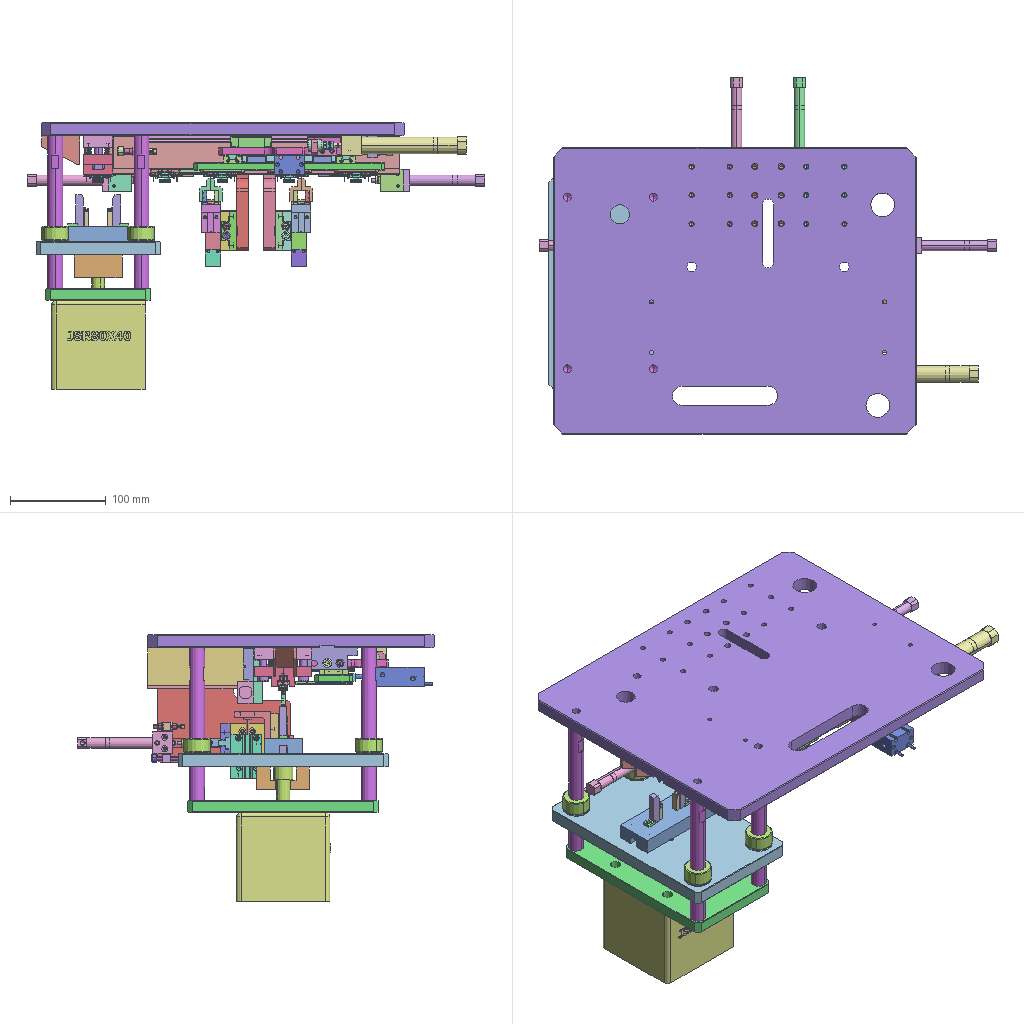Assembly | STEP file | 119 different items | 282 placed | box 479 x 373 x 279 mm
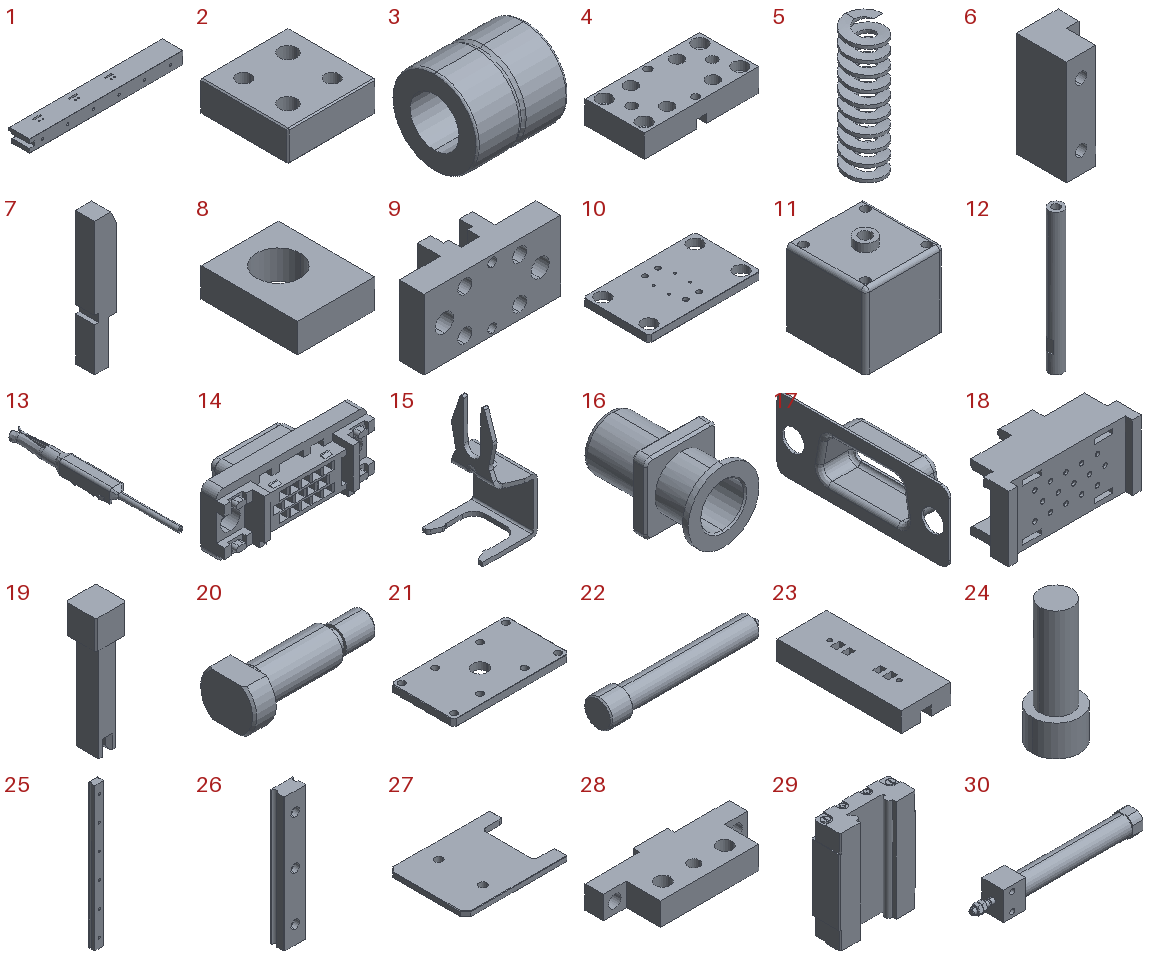Parts list (item | name | quantity | parent item | size | volume):
1 | Semi-finished track | x1 | in Assembly | 300 x 40 x 24 mm | 231580 mm3
2 | A037 | x2 | in Assembly | 20 x 20 x 7 mm | 2500 mm3
3 | LMUT16 | x4 | in Riveting rivet station | 29.9 x 28 x 28 mm | 12313 mm3
4 | Riveting base | x1 | in Riveting rivet station | 60 x 30.8 x 12 mm | 18745 mm3
5 | SWF6-20 spring | x4 | in Riveting rivet station | 6 x 6 x 20 mm | 104.246 mm3
6 | Large cylinder connector mounting block | x2 | in Riveting rivet station | 20 x 24 x 50 mm | 18141 mm3
7 | Riveting product locating pin | x2 | in Riveting rivet station | 8 x 7 x 49 mm | 2346 mm3
8 | Stopper plate | x2 | in Riveting rivet station | 8 x 10 x 3 mm | 192.287 mm3
9 | Riveting floating block | x1 | in Riveting rivet station | 60 x 20.8 x 30.8 mm | 21870 mm3
10 | Riveting slide mounting plate | x1 | in Riveting rivet station | 220 x 130 x 14 mm | 361910 mm3
11 | JSR80X40 | x1 | in Riveting rivet station | 99 x 98 x 103.5 mm | 861667 mm3
12 | Guide pillar | x4 | in Riveting rivet station | 16 x 16 x 160 mm | 28723 mm3
13 | CONTACT | x75 | - | 1.85 x 19.165 x 1.65 mm | 9.871 mm3
14 | HOUSING | x5 | - | 30.8 x 13.55 x 12.55 mm | 1641 mm3
15 | LATCH | x10 | - | 4.62 x 5.1 x 10 mm | 18.37 mm3
16 | MAODING | x10 | - | 5 x 8 x 5 mm | 51.782 mm3
17 | SHELL | x5 | - | 6.2 x 30.8 x 12.55 mm | 200.201 mm3
18 | COVER | x5 | - | 19.4 x 8.9 x 9.6 mm | 433.37 mm3
19 | Riveting press block | x2 | in Riveting rivet station | 8.5 x 8.5 x 35.35 mm | 1342 mm3
20 | CLBDG8-18 | x2 | in Riveting rivet station | 32 x 13 x 10 mm | 1712 mm3
21 | Large cylinder base plate | x1 | in Riveting rivet station | 200 x 110 x 12 mm | 247760 mm3
22 | Riveting punch | x2 | in Riveting rivet station | 28.754 x 5 x 5 mm | 342.473 mm3
23 | Riveting upper die seat | x1 | in Riveting rivet station | 40 x 100 x 16 mm | 55230 mm3
24 | M14 screw | x1 | in Riveting rivet station | 20.67 x 20.67 x 53.57 mm | 10711 mm3
25 | 1SE2BZ16-230 | x1 | in Assembly | 15 x 9.5 x 230 mm | 29723 mm3
26 | SEBZ10-551 | x2 | in Assembly | 9 x 5.5 x 55 mm | 2176 mm3
27 | A039 | x2 | in Assembly | 60 x 46 x 3 mm | 7033 mm3
28 | Stopper buffer seat | x2 | in Assembly | 63 x 26 x 10 mm | 10700 mm3
29 | 2SE2BZ16-230 | x1 | in Assembly | 32 x 12 x 42.4 mm | 12424 mm3
30 | CJ2RA16-75(0_0_0) | x1 | in Assembly | - | -
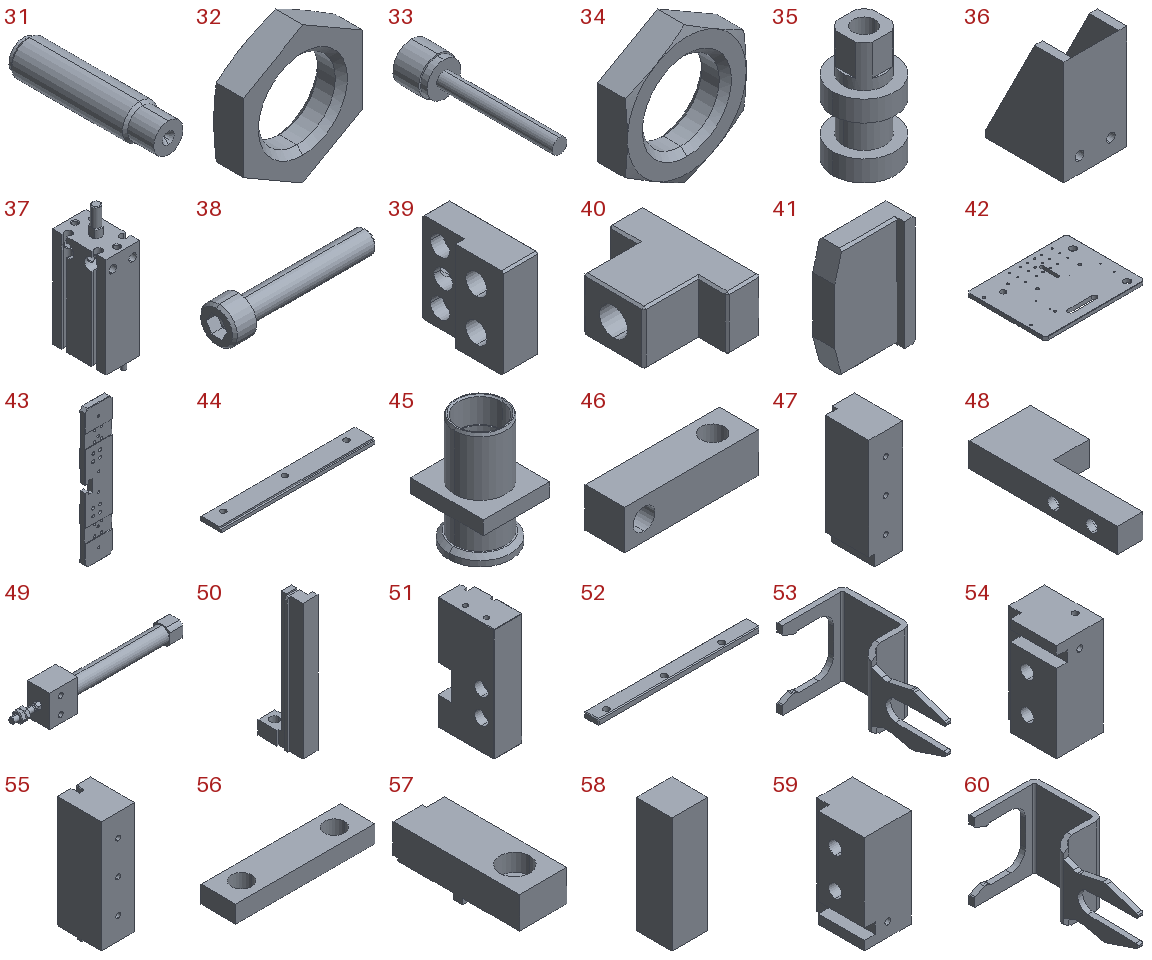31 | MAKC0604A1 | x4 | in MAKC0604A | 6 x 25 x 6 mm | 609.83 mm3
32 | MAKC0604A4 | x4 | in MAKC0604A | 8 x 2 x 9.238 mm | 65.48 mm3
33 | MAKC0604A2 | x4 | in MAKC0604A | 4.6 x 18.25 x 4.6 mm | 100.526 mm3
34 | MAKC0604A3 | x4 | in MAKC0604A | 8 x 2 x 9.238 mm | 65.48 mm3
35 | Product shift T-head | x1 | in Assembly | 12 x 12 x 22 mm | 1377 mm3
36 | Discharge hopper | x1 | in Assembly | 24 x 30 x 40 mm | 12073 mm3
37 | CDU16-20D-A93 (0) | x1 | in Assembly | 20 x 32 x 85 mm | 33757 mm3
38 | CB6-35 | x2 | in Assembly | 41 x 10 x 10 mm | 1382 mm3
39 | Brake spring-press seat | x3 | in Assembly | 6 x 15 x 15 mm | 832.507 mm3
40 | A036 | x1 | in Assembly | 13 x 17.5 x 8 mm | 1094 mm3
41 | Brake block | x3 | in Assembly | 10 x 4 x 15 mm | 442.73 mm3
42 | Base plate | x1 | in Assembly | 380 x 300 x 14 mm | 1501141 mm3
43 | A034 | x1 | in Assembly | 40 x 8 x 200 mm | 52528 mm3
44 | Feed slide cover_Default | x2 | in Rivet-harpoon feed and assembly | 100 x 13 x 3 mm | 3712 mm3
45 | Rivet_Default | x3 | in Rivet-harpoon feed and assembly | 4.8 x 5.3 x 8.1 mm | 41.537 mm3
46 | Optical fiber mount | x1 | in Rivet-harpoon feed and assembly | 20.5 x 6 x 6 mm | 628.955 mm3
47 | Harpoon feed slide_Default | x1 | in Rivet-harpoon feed and assembly | 30 x 42.8 x 100 mm | 120679 mm3
48 | Rivet air-suction cylinder seat | x1 | in Rivet-harpoon feed and assembly | 24 x 58 x 9.55 mm | 7786 mm3
49 | CJ2RKA10-45(0_0_0) | x2 | in Rivet-harpoon feed and assembly, Rivet-harpoon shift assembly | - | -
50 | Rivet push rod_Default | x1 | in Rivet-harpoon feed and assembly | 6.34 x 16 x 50 mm | 1914 mm3
51 | Rivet push-in slide_Default | x1 | in Rivet-harpoon feed and assembly | 20 x 40 x 80 mm | 57141 mm3
52 | Harpoon track cover plate_Default | x1 | in Rivet-harpoon feed and assembly | 98 x 8.5 x 3.6 mm | 2841 mm3
53 | Harpoon_Default | x2 | in Rivet-harpoon feed and assembly | 4.47 x 10 x 5.3 mm | 19.521 mm3
54 | Rivet press-in harpoon track_Default | x1 | in Rivet-harpoon feed and assembly | 20 x 25 x 42 mm | 18009 mm3
55 | Rivet feed slide_Default | x1 | in Rivet-harpoon feed and assembly | 30 x 39.6 x 101.8 mm | 114670 mm3
56 | Spring stop block | x3 | in Rivet-harpoon feed and assembly, Mirror rivet-harpoon feed and assembly, Assembly | 24 x 6 x 3 mm | 374.273 mm3
57 | Rivet push-in slide2_Default | x1 | in Rivet-harpoon feed and assembly | 15 x 40 x 11.8 mm | 5491 mm3
58 | Harpoon track spring pin | x1 | in Rivet-harpoon feed and assembly | 4.58 x 4.58 x 15 mm | 314.646 mm3
59 | Mirror rivet press-in harpoon track_Default | x1 | in Mirror rivet-harpoon feed and assembly | 20 x 25 x 42 mm | 18009 mm3
60 | Mirror harpoon_Default | x2 | in Mirror rivet-harpoon feed and assembly | 4.47 x 10 x 5.3 mm | 19.521 mm3
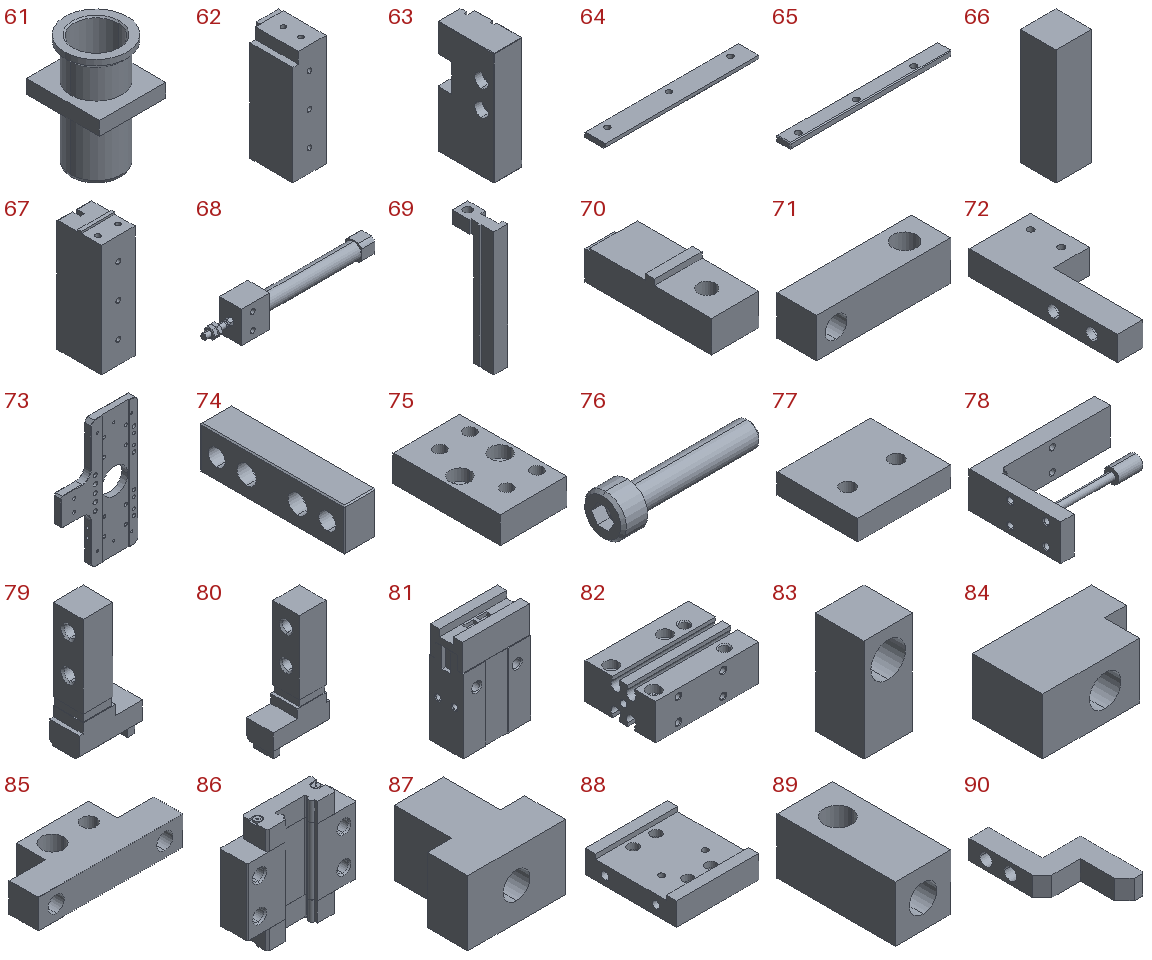61 | Mirror rivet_Default | x3 | in Mirror rivet-harpoon feed and assembly | 4.8 x 5.3 x 8.1 mm | 41.537 mm3
62 | Mirror harpoon feed slide_Default | x1 | in Mirror rivet-harpoon feed and assembly | 30 x 42.8 x 100 mm | 120679 mm3
63 | Mirror rivet push-in slide_Default | x1 | in Mirror rivet-harpoon feed and assembly | 20 x 40 x 80 mm | 57141 mm3
64 | Mirror feed slide cover_Default | x2 | in Mirror rivet-harpoon feed and assembly | 100 x 13 x 3 mm | 3712 mm3
65 | Mirror harpoon track cover plate_Default | x1 | in Mirror rivet-harpoon feed and assembly | 98 x 8.5 x 3.6 mm | 2841 mm3
66 | Mirror harpoon track spring pin | x1 | in Mirror rivet-harpoon feed and assembly | 4.58 x 4.58 x 15 mm | 314.646 mm3
67 | Mirror rivet feed slide_Default | x1 | in Mirror rivet-harpoon feed and assembly | 30 x 39.6 x 101.8 mm | 114670 mm3
68 | Mirror CJ2RKA10-45(0_0_0) | x1 | in Mirror rivet-harpoon feed and assembly | 119 x 16 x 23 mm | 12263 mm3
69 | Mirror rivet push rod_Default | x1 | in Mirror rivet-harpoon feed and assembly | 6.34 x 16 x 50 mm | 1914 mm3
70 | Mirror rivet push-in slide2_Default | x1 | in Mirror rivet-harpoon feed and assembly | 15 x 40 x 11.8 mm | 5491 mm3
71 | Mirror optical fiber mount | x1 | in Mirror rivet-harpoon feed and assembly | 20.5 x 6 x 6 mm | 628.955 mm3
72 | Mirror rivet air-suction cylinder seat | x1 | in Mirror rivet-harpoon feed and assembly | 24 x 58 x 9.55 mm | 7786 mm3
73 | A033 | x1 | in Assembly | 90 x 8 x 148 mm | 59811 mm3
74 | A038 | x2 | in Assembly | 7.5 x 34 x 10 mm | 1805 mm3
75 | Gripper cylinder connecting plate | x1 | in Rivet-harpoon shift assembly | 20 x 32 x 8 mm | 4330 mm3
76 | CBAL5-25 | x2 | in Rivet-harpoon shift assembly | 30 x 8.5 x 8.5 mm | 731.85 mm3
77 | Shift cylinder pad | x1 | in Rivet-harpoon shift assembly | 23 x 20 x 5 mm | 2204 mm3
78 | MXH6-15-b | x1 | in Rivet-harpoon shift assembly | 52 x 38 x 15 mm | 8036 mm3
79 | 2 | x1 | in MHZA2-6D | 8.45 x 4 x 17.2 mm | 295.775 mm3
80 | 3 | x1 | in MHZA2-6D | 8.45 x 4 x 17.2 mm | 295.775 mm3
81 | 1 | x1 | in MHZA2-6D | 20 x 10 x 29.8 mm | 5405 mm3
82 | MXH6-15-a | x1 | in Rivet-harpoon shift assembly | 46 x 31.7 x 16 mm | 17954 mm3
83 | Buffer mount | x1 | in Rivet-harpoon shift assembly | 8.5 x 8.5 x 18 mm | 935.428 mm3
84 | Shift T-head fixing seat | x2 | in Rivet-harpoon shift assembly | 16.9 x 10 x 8 mm | 941.722 mm3
85 | Harpoon shift buffer fixing seat | x1 | in Rivet-harpoon shift assembly | 40 x 16 x 8 mm | 2986 mm3
86 | Linear slider | x1 | in Rivet-harpoon shift assembly | 31 x 7.8 x 30 mm | 4960 mm3
87 | Shift T-type connector | x1 | in Rivet-harpoon shift assembly | 12 x 12 x 8 mm | 713.364 mm3
88 | Slide cylinder mount | x1 | in Rivet-harpoon shift assembly | 36 x 40 x 10 mm | 10816 mm3
89 | Stopper | x1 | in Rivet-harpoon shift assembly | 8.5 x 18 x 8.5 mm | 1038 mm3
90 | Gripper_Default | x2 | in Rivet-harpoon shift assembly | 11.85 x 24 x 4 mm | 454.253 mm3
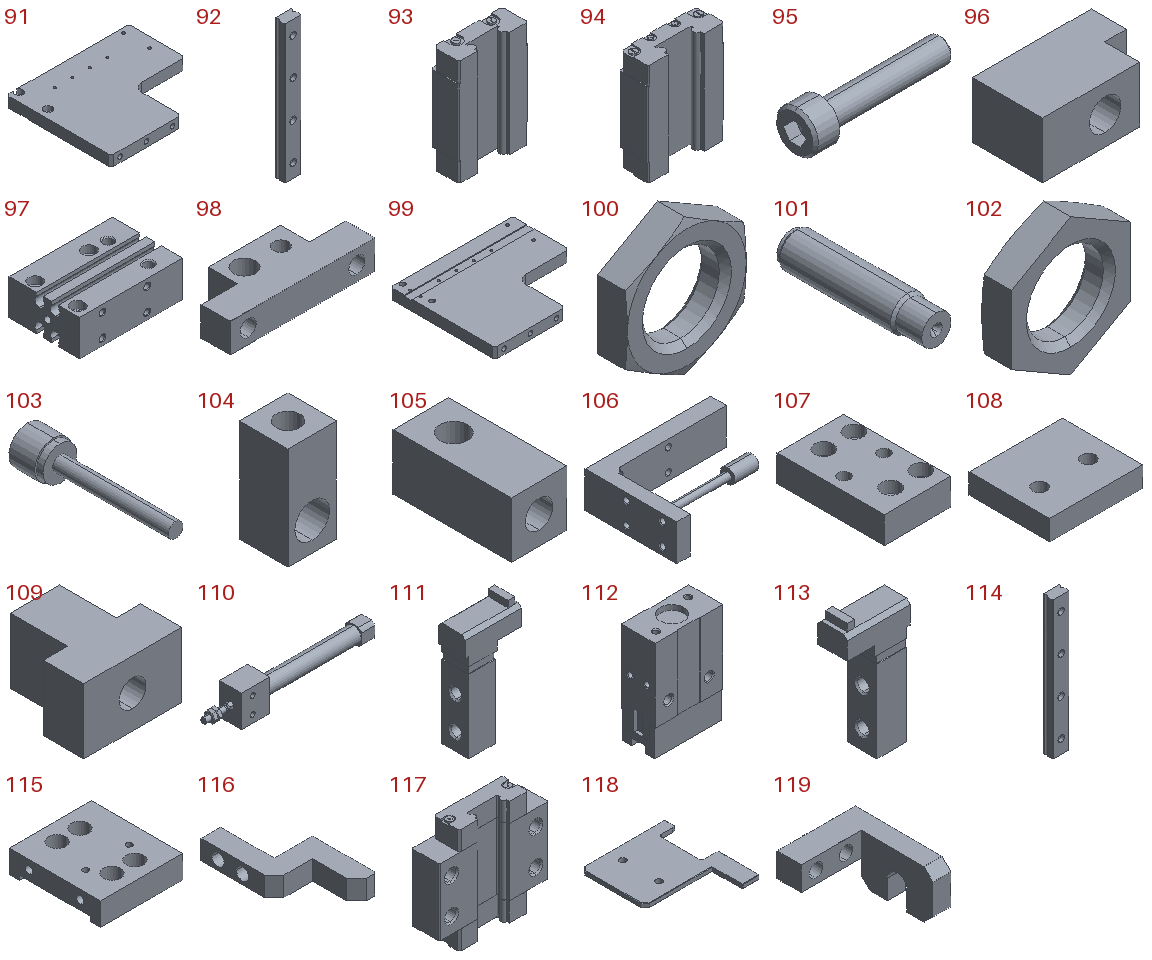91 | Shift support plate_Default | x1 | in Rivet-harpoon shift assembly | 140 x 120 x 12 mm | 158109 mm3
92 | Linear rail | x1 | in Rivet-harpoon shift assembly | 9 x 5.5 x 75 mm | 3056 mm3
93 | SEBZ10-552 | x2 | in Assembly | 20 x 7.8 x 30 mm | 3537 mm3
94 | 3SE2BZ16-230 | x1 | in Assembly | 32 x 12 x 42.4 mm | 12424 mm3
95 | Mirror CBAL5-25 | x2 | in Mirror rivet-harpoon shift assembly | 30 x 8.5 x 8.5 mm | 731.85 mm3
96 | Mirror shift T-head fixing seat | x2 | in Mirror rivet-harpoon shift assembly | 16.9 x 10 x 8 mm | 941.722 mm3
97 | Mirror MXH6-15-a | x1 | in Mirror rivet-harpoon shift assembly | 46 x 31.7 x 16 mm | 17954 mm3
98 | Mirror harpoon shift buffer fixing seat | x1 | in Mirror rivet-harpoon shift assembly | 40 x 16 x 8 mm | 2986 mm3
99 | Mirror shift support plate_Default | x1 | in Mirror rivet-harpoon shift assembly | 140 x 120 x 12 mm | 158109 mm3
100 | Mirror MAKC0604A3 | x2 | in 101, Mirror MAKC0604A | 8 x 2 x 9.238 mm | 65.48 mm3
101 | Mirror MAKC0604A1 | x2 | in 101, Mirror MAKC0604A | 6 x 25 x 6 mm | 609.83 mm3
102 | Mirror MAKC0604A4 | x2 | in 101, Mirror MAKC0604A | 8 x 2 x 9.238 mm | 65.48 mm3
103 | Mirror MAKC0604A2 | x2 | in 101, Mirror MAKC0604A | 4.6 x 18.25 x 4.6 mm | 100.526 mm3
104 | Mirror buffer mount | x1 | in Mirror rivet-harpoon shift assembly | 8.5 x 8.5 x 18 mm | 935.428 mm3
105 | Mirror stopper | x1 | in Mirror rivet-harpoon shift assembly | 8.5 x 18 x 8.5 mm | 1038 mm3
106 | Mirror MXH6-15-b | x1 | in Mirror rivet-harpoon shift assembly | 52 x 38 x 15 mm | 8036 mm3
107 | Mirror gripper cylinder connecting plate | x1 | in Mirror rivet-harpoon shift assembly | 20 x 32 x 8 mm | 4330 mm3
108 | Mirror shift cylinder pad | x1 | in Mirror rivet-harpoon shift assembly | 23 x 20 x 5 mm | 2204 mm3
109 | Mirror shift T-type connector | x1 | in Mirror rivet-harpoon shift assembly | 12 x 12 x 8 mm | 713.364 mm3
110 | Mirror CJ2RKA10-45(0_0_0)1 | x1 | in Mirror rivet-harpoon shift assembly | 119 x 16 x 23 mm | 12263 mm3
111 | Mirror2 | x1 | in Mirror MHZA2-6D | 8.45 x 4 x 17.2 mm | 295.775 mm3
112 | Mirror1 | x1 | in Mirror MHZA2-6D | 20 x 10 x 29.8 mm | 5405 mm3
113 | Mirror3 | x1 | in Mirror MHZA2-6D | 8.45 x 4 x 17.2 mm | 295.775 mm3
114 | Mirror linear rail | x1 | in Mirror rivet-harpoon shift assembly | 9 x 5.5 x 75 mm | 3056 mm3
115 | Mirror slide cylinder mount | x1 | in Mirror rivet-harpoon shift assembly | 36 x 40 x 10 mm | 10816 mm3
116 | Mirror gripper_Default | x2 | in Mirror rivet-harpoon shift assembly | 11.85 x 24 x 4 mm | 454.253 mm3
117 | Mirror linear slider | x1 | in Mirror rivet-harpoon shift assembly | 31 x 7.8 x 30 mm | 4960 mm3
118 | Riveting station pick claw | x1 | in Assembly | 60 x 67.74 x 3 mm | 7814 mm3
119 | Product shift cylinder connector | x1 | in Assembly | 26 x 32 x 16 mm | 3279 mm3
Placements (level | parent | child | x y z in mm | rotation matrix by rows):
1 | Assembly | Semi-finished track | -101.117 -51.384 -17.0 | 1 0 0 0 0 1 0 -1 0
1 | Assembly | A037 | 33.992 -10.639 -35.0 | -1 0 0 0 -1 0 0 0 1
1 | Assembly | Riveting rivet station | -113.758 -35.953 -13.0 | 0 -1 0 -1 0 0 0 0 -1
2 | Riveting rivet station | LMUT16 | -86.569 -42.241 118.75 | 0 -0.8149 0.5796 0 0.5796 0.8149 -1 0 0
2 | Riveting rivet station | Riveting base | -26.539 -12.691 -6.0 | 1 0 0 0 1 0 0 0 1
2 | Riveting rivet station | SWF6-20 spring | -8.595 -6.448 -1.8 | 0.2253 0.9743 0 -0.9743 0.2253 0 0 0 1
2 | Riveting rivet station | Large cylinder connector mounting block | -4.069 27.759 118.65 | 1 0 0 0 0 -1 0 1 -0
2 | Riveting rivet station | Riveting product locating pin | 7.931 26.204 104.65 | 0 -1 0 -1 0 0 0 0 -1
2 | Riveting rivet station | Stopper plate | 7.931 -21.612 85.65 | -1 0 0 0 -1 0 0 0 1
2 | Riveting rivet station | Riveting floating block | -26.539 18.109 14.0 | 1 0 0 0 0 -1 0 1 0
2 | Riveting rivet station | Riveting slide mounting plate | -106.569 -62.241 104.65 | 1 0 0 0 1 0 0 0 1
2 | Riveting rivet station | Stopper plate | -0.069 27.129 85.65 | 1 0 0 0 1 0 0 0 1
2 | Riveting rivet station | Riveting product locating pin | -1.069 -20.686 104.65 | 0 1 0 1 0 0 0 0 -1
2 | Riveting rivet station | JSR80X40 | 3.431 2.759 210.5 | 1 0 0 0 -1 0 0 0 -1
2 | Riveting rivet station | LMUT16 | 93.431 -42.241 118.75 | 0 -0.8149 0.5796 0 0.5796 0.8149 -1 0 0
2 | Riveting rivet station | Guide pillar | -86.569 -42.241 -6.0 | 1 0 0 0 1 0 0 0 1
2 | Riveting rivet station | SWF6-20 spring | 15.405 12.352 -1.8 | 0.2253 0.9743 0 -0.9743 0.2253 0 0 0 1
2 | Riveting rivet station | subassembly 2 | 9.711 18.109 36.35 | 0 0 1 -1 0 0 0 -1 0
3 | subassembly 2 | CONTACT | 20.235 -6.585 -8.205 | 1 0 0 0 1 0 0 0 1
3 | subassembly 2 | CONTACT | 12.22 -6.585 -6.225 | 1 0 0 0 1 0 0 0 1
3 | subassembly 2 | HOUSING | 15.4 7.3 -6.275 | 1 0 0 0 1 0 0 0 1
3 | subassembly 2 | CONTACT | 16.8 -6.585 -6.225 | 1 0 0 0 1 0 0 0 1
3 | subassembly 2 | CONTACT | 15.655 -6.585 -4.245 | 1 0 0 0 1 0 0 0 1
3 | subassembly 2 | LATCH | 2.73 -0.15 -6.275 | 1 0 0 0 0 -1 0 1 0
3 | subassembly 2 | CONTACT | 14.51 -6.585 -6.225 | 1 0 0 0 1 0 0 0 1
3 | subassembly 2 | CONTACT | 9.93 -6.585 -6.225 | 1 0 0 0 1 0 0 0 1
3 | subassembly 2 | CONTACT | 13.365 -6.585 -4.245 | 1 0 0 0 1 0 0 0 1
3 | subassembly 2 | CONTACT | 19.09 -6.585 -6.225 | 1 0 0 0 1 0 0 0 1
3 | subassembly 2 | MAODING | 27.895 -0.15 -6.275 | 1 0 0 0 1 0 0 0 1
3 | subassembly 2 | SHELL | 15.4 7.7 -10.275 | 0 1 0 1 0 0 0 0 -1
3 | subassembly 2 | CONTACT | 11.075 -6.585 -4.245 | 1 0 0 0 1 0 0 0 1
3 | subassembly 2 | CONTACT | 17.945 -6.585 -8.205 | 1 0 0 0 1 0 0 0 1
3 | subassembly 2 | CONTACT | 11.075 -6.585 -8.205 | 1 0 0 0 1 0 0 0 1
3 | subassembly 2 | CONTACT | 20.235 -6.585 -4.245 | 1 0 0 0 1 0 0 0 1
3 | subassembly 2 | MAODING | 2.905 -0.15 -6.275 | 1 0 0 0 1 0 0 0 1
3 | subassembly 2 | CONTACT | 13.365 -6.585 -8.205 | 1 0 0 0 1 0 0 0 1
3 | subassembly 2 | COVER | 15.4 -1.6 -6.275 | -1 0 0 0 1 0 0 0 -1
3 | subassembly 2 | CONTACT | 15.655 -6.585 -8.205 | 1 0 0 0 1 0 0 0 1
3 | subassembly 2 | CONTACT | 17.945 -6.585 -4.245 | 1 0 0 0 1 0 0 0 1
3 | subassembly 2 | LATCH | 28.07 -0.15 -6.275 | -1 0 0 0 0 -1 0 -1 0
2 | Riveting rivet station | Riveting press block | 3.431 -9.736 94.65 | 0 -1 0 1 0 0 0 0 1
2 | Riveting rivet station | LMUT16 | 93.431 47.759 118.75 | 0 -0.8253 0.5646 0 0.5646 0.8253 -1 0 0
2 | Riveting rivet station | CLBDG8-18 | 24.461 2.709 24.0 | 0 0.09473 0.9955 0 0.9955 -0.09473 -1 0 0
2 | Riveting rivet station | Riveting press block | 3.431 15.254 94.65 | 0 1 0 -1 0 0 0 0 1
2 | Riveting rivet station | LMUT16 | -86.569 47.759 118.75 | 0 -0.2367 0.9716 0 0.9716 0.2367 -1 0 0
2 | Riveting rivet station | Guide pillar | 93.431 47.759 -6.0 | 1 0 0 0 1 0 0 0 1
2 | Riveting rivet station | CLBDG8-18 | -17.539 2.709 24.0 | 0 0.18 0.9837 0 0.9837 -0.18 -1 0 0
2 | Riveting rivet station | SWF6-20 spring | -8.595 12.352 -1.8 | 0.2253 0.9743 0 -0.9743 0.2253 0 0 0 1
2 | Riveting rivet station | Guide pillar | 93.431 -42.241 -6.0 | 1 0 0 0 1 0 0 0 1
2 | Riveting rivet station | Large cylinder base plate | -96.569 -52.241 154.0 | 1 0 0 0 1 0 0 0 1
2 | Riveting rivet station | Riveting punch | 37.701 -11.606 -17357.62 | 0 -0.9986 -0.05276 0 0.05276 -0.9986 1 0 -0
2 | Riveting rivet station | SWF6-20 spring | 15.405 -6.448 -1.8 | 0.2253 0.9743 0 -0.9743 0.2253 0 0 0 1
2 | Riveting rivet station | Riveting upper die seat | -16.569 22.759 104.65 | 1 0 0 0 -1 0 0 0 -1
2 | Riveting rivet station | Guide pillar | -86.569 47.759 -6.0 | 1 0 0 0 1 0 0 0 1
2 | Riveting rivet station | Riveting punch | 21.022 -14.308 -17357.62 | 0 -0.5136 -0.858 0 0.858 -0.5136 1 0 0
2 | Riveting rivet station | M14 screw | 3.431 2.759 118.65 | 0.9149 0.4037 0 -0.4037 0.9149 0 0 0 1
2 | Riveting rivet station | Large cylinder connector mounting block | 10.931 -22.241 118.65 | -1 0 0 0 0 1 0 1 0
1 | Assembly | 1SE2BZ16-230 | -66.322 -85.484 -4.0 | 0 0 1 -1 0 0 0 -1 0
1 | Assembly | subassembly 2 | -61.872 -45.709 -49.0 | 1 0 0 0 0 -1 0 1 -0
2 | subassembly 2 | CONTACT | 20.235 -6.585 -8.205 | 1 0 0 0 1 0 0 0 1
2 | subassembly 2 | CONTACT | 12.22 -6.585 -6.225 | 1 0 0 0 1 0 0 0 1
2 | subassembly 2 | HOUSING | 15.4 7.3 -6.275 | 1 0 0 0 1 0 0 0 1
2 | subassembly 2 | CONTACT | 16.8 -6.585 -6.225 | 1 0 0 0 1 0 0 0 1
2 | subassembly 2 | CONTACT | 15.655 -6.585 -4.245 | 1 0 0 0 1 0 0 0 1
2 | subassembly 2 | LATCH | 2.73 -0.15 -6.275 | 1 0 0 0 0 -1 0 1 0
2 | subassembly 2 | CONTACT | 14.51 -6.585 -6.225 | 1 0 0 0 1 0 0 0 1
2 | subassembly 2 | CONTACT | 9.93 -6.585 -6.225 | 1 0 0 0 1 0 0 0 1
2 | subassembly 2 | CONTACT | 13.365 -6.585 -4.245 | 1 0 0 0 1 0 0 0 1
2 | subassembly 2 | CONTACT | 19.09 -6.585 -6.225 | 1 0 0 0 1 0 0 0 1
2 | subassembly 2 | MAODING | 27.895 -0.15 -6.275 | 1 0 0 0 1 0 0 0 1
2 | subassembly 2 | SHELL | 15.4 7.7 -10.275 | 0 1 0 1 0 0 0 0 -1
2 | subassembly 2 | CONTACT | 11.075 -6.585 -4.245 | 1 0 0 0 1 0 0 0 1
2 | subassembly 2 | CONTACT | 17.945 -6.585 -8.205 | 1 0 0 0 1 0 0 0 1
2 | subassembly 2 | CONTACT | 11.075 -6.585 -8.205 | 1 0 0 0 1 0 0 0 1
2 | subassembly 2 | CONTACT | 20.235 -6.585 -4.245 | 1 0 0 0 1 0 0 0 1
2 | subassembly 2 | MAODING | 2.905 -0.15 -6.275 | 1 0 0 0 1 0 0 0 1
2 | subassembly 2 | CONTACT | 13.365 -6.585 -8.205 | 1 0 0 0 1 0 0 0 1
2 | subassembly 2 | COVER | 15.4 -1.6 -6.275 | -1 0 0 0 1 0 0 0 -1
2 | subassembly 2 | CONTACT | 15.655 -6.585 -8.205 | 1 0 0 0 1 0 0 0 1
2 | subassembly 2 | CONTACT | 17.945 -6.585 -4.245 | 1 0 0 0 1 0 0 0 1
2 | subassembly 2 | LATCH | 28.07 -0.15 -6.275 | -1 0 0 0 0 -1 0 -1 0
1 | Assembly | SEBZ10-551 | 143.173 -59.484 -26.0 | -1 0 0 0 0 -1 0 -1 -0
1 | Assembly | A039 | 106.673 -135.763 -45.0 | 0 -1 0 1 0 0 0 0 1
1 | Assembly | Stopper buffer seat | 175.678 -61.984 -30.0 | 0 0 -1 -1 0 0 0 1 -0
1 | Assembly | 2SE2BZ16-230 | -97.527 -85.484 -4.0 | 0 0 1 -1 0 0 0 -1 -0
1 | Assembly | SEBZ10-551 | 24.173 -59.484 -26.0 | -1 0 0 0 0 -1 0 -1 -0
1 | Assembly | CJ2RA16-75(0_0_0) | 138.678 -134.484 -17.0 | 1 0 0 0 0 1 0 -1 0
1 | Assembly | MAKC0604A | 178.282 -93.785 -17.461 | 0 -1 0 0.9964 0 -0.08483 0.08483 0 0.9964
2 | MAKC0604A | MAKC0604A1 | -5.65 -3.2 -5.078 | 1 0 0 0 1 0 0 0 1
2 | MAKC0604A | MAKC0604A4 | -5.65 -4.772 -5.078 | 1 0 0 0 1 0 0 0 1
2 | MAKC0604A | MAKC0604A2 | -5.65 -3.246 -5.078 | 1 0 0 0 1 0 0 0 1
2 | MAKC0604A | MAKC0604A3 | -5.65 -2.522 -5.078 | 1 0 0 0 1 0 0 0 1
1 | Assembly | Stopper buffer seat | -68.322 -61.984 -30.0 | 0 0 -1 -1 0 0 0 1 -0
1 | Assembly | Product shift T-head | 103.368 -134.484 -17.0 | 0 0 1 0.2721 0.9623 0 -0.9623 0.2721 0
1 | Assembly | Discharge hopper | -135.749 -52.914 -7.0 | 0 0 -1 1 0 0 0 -1 -0
1 | Assembly | CDU16-20D-A93 (0) | 83.673 -126.984 -37.0 | 0 -1 0 0 0 1 -1 0 0
1 | Assembly | CB6-35 | 185.811 -85.484 -23.0 | -1 0 0 0 -0.9638 -0.2667 0 -0.2667 0.9638
1 | Assembly | subassembly 2 | -1.727 -45.709 -49.0 | 1 0 0 0 0 -1 0 1 -0
2 | subassembly 2 | CONTACT | 20.235 -6.585 -8.205 | 1 0 0 0 1 0 0 0 1
2 | subassembly 2 | CONTACT | 12.22 -6.585 -6.225 | 1 0 0 0 1 0 0 0 1
2 | subassembly 2 | HOUSING | 15.4 7.3 -6.275 | 1 0 0 0 1 0 0 0 1
2 | subassembly 2 | CONTACT | 16.8 -6.585 -6.225 | 1 0 0 0 1 0 0 0 1
2 | subassembly 2 | CONTACT | 15.655 -6.585 -4.245 | 1 0 0 0 1 0 0 0 1
2 | subassembly 2 | LATCH | 2.73 -0.15 -6.275 | 1 0 0 0 0 -1 0 1 0
2 | subassembly 2 | CONTACT | 14.51 -6.585 -6.225 | 1 0 0 0 1 0 0 0 1
2 | subassembly 2 | CONTACT | 9.93 -6.585 -6.225 | 1 0 0 0 1 0 0 0 1
2 | subassembly 2 | CONTACT | 13.365 -6.585 -4.245 | 1 0 0 0 1 0 0 0 1
2 | subassembly 2 | CONTACT | 19.09 -6.585 -6.225 | 1 0 0 0 1 0 0 0 1
2 | subassembly 2 | MAODING | 27.895 -0.15 -6.275 | 1 0 0 0 1 0 0 0 1
2 | subassembly 2 | SHELL | 15.4 7.7 -10.275 | 0 1 0 1 0 0 0 0 -1
2 | subassembly 2 | CONTACT | 11.075 -6.585 -4.245 | 1 0 0 0 1 0 0 0 1
2 | subassembly 2 | CONTACT | 17.945 -6.585 -8.205 | 1 0 0 0 1 0 0 0 1
2 | subassembly 2 | CONTACT | 11.075 -6.585 -8.205 | 1 0 0 0 1 0 0 0 1
2 | subassembly 2 | CONTACT | 20.235 -6.585 -4.245 | 1 0 0 0 1 0 0 0 1
2 | subassembly 2 | MAODING | 2.905 -0.15 -6.275 | 1 0 0 0 1 0 0 0 1
2 | subassembly 2 | CONTACT | 13.365 -6.585 -8.205 | 1 0 0 0 1 0 0 0 1
2 | subassembly 2 | COVER | 15.4 -1.6 -6.275 | -1 0 0 0 1 0 0 0 -1
2 | subassembly 2 | CONTACT | 15.655 -6.585 -8.205 | 1 0 0 0 1 0 0 0 1
2 | subassembly 2 | CONTACT | 17.945 -6.585 -4.245 | 1 0 0 0 1 0 0 0 1
2 | subassembly 2 | LATCH | 28.07 -0.15 -6.275 | -1 0 0 0 0 -1 0 -1 0
1 | Assembly | CB6-35 | -90.194 -85.484 -23.0 | 1 0 0 0 -0.1791 -0.9838 0 0.9838 -0.1791
1 | Assembly | Brake spring-press seat | 90.883 -37.965 -37.463 | 0 0 -1 1 0 0 0 -1 0
1 | Assembly | A036 | 93.153 -118.356 -42.0 | 0 -1 0 1 0 0 0 0 1
1 | Assembly | Brake block | -49.117 -57.945 -35.789 | 0 0 -1 1 0 0 0 -1 0
1 | Assembly | subassembly 2 | 138.273 -45.709 -49.0 | 1 0 0 0 0 -1 0 1 -0
2 | subassembly 2 | CONTACT | 20.235 -6.585 -8.205 | 1 0 0 0 1 0 0 0 1
2 | subassembly 2 | CONTACT | 12.22 -6.585 -6.225 | 1 0 0 0 1 0 0 0 1
2 | subassembly 2 | HOUSING | 15.4 7.3 -6.275 | 1 0 0 0 1 0 0 0 1
2 | subassembly 2 | CONTACT | 16.8 -6.585 -6.225 | 1 0 0 0 1 0 0 0 1
2 | subassembly 2 | CONTACT | 15.655 -6.585 -4.245 | 1 0 0 0 1 0 0 0 1
2 | subassembly 2 | LATCH | 2.73 -0.15 -6.275 | 1 0 0 0 0 -1 0 1 0
2 | subassembly 2 | CONTACT | 14.51 -6.585 -6.225 | 1 0 0 0 1 0 0 0 1
2 | subassembly 2 | CONTACT | 9.93 -6.585 -6.225 | 1 0 0 0 1 0 0 0 1
2 | subassembly 2 | CONTACT | 13.365 -6.585 -4.245 | 1 0 0 0 1 0 0 0 1
2 | subassembly 2 | CONTACT | 19.09 -6.585 -6.225 | 1 0 0 0 1 0 0 0 1
2 | subassembly 2 | MAODING | 27.895 -0.15 -6.275 | 1 0 0 0 1 0 0 0 1
2 | subassembly 2 | SHELL | 15.4 7.7 -10.275 | 0 1 0 1 0 0 0 0 -1
2 | subassembly 2 | CONTACT | 11.075 -6.585 -4.245 | 1 0 0 0 1 0 0 0 1
2 | subassembly 2 | CONTACT | 17.945 -6.585 -8.205 | 1 0 0 0 1 0 0 0 1
2 | subassembly 2 | CONTACT | 11.075 -6.585 -8.205 | 1 0 0 0 1 0 0 0 1
2 | subassembly 2 | CONTACT | 20.235 -6.585 -4.245 | 1 0 0 0 1 0 0 0 1
2 | subassembly 2 | MAODING | 2.905 -0.15 -6.275 | 1 0 0 0 1 0 0 0 1
2 | subassembly 2 | CONTACT | 13.365 -6.585 -8.205 | 1 0 0 0 1 0 0 0 1
2 | subassembly 2 | COVER | 15.4 -1.6 -6.275 | -1 0 0 0 1 0 0 0 -1
2 | subassembly 2 | CONTACT | 15.655 -6.585 -8.205 | 1 0 0 0 1 0 0 0 1
2 | subassembly 2 | CONTACT | 17.945 -6.585 -4.245 | 1 0 0 0 1 0 0 0 1
2 | subassembly 2 | LATCH | 28.07 -0.15 -6.275 | -1 0 0 0 0 -1 0 -1 0
1 | Assembly | Base plate | -196.322 -197.484 -7.0 | 1 0 0 0 1 0 0 0 1
1 | Assembly | A034 | 183.673 -78.657 -48.98 | 0 0 -1 1 0 0 0 -1 0
1 | Assembly | A037 | 203.019 -80.303 -35.0 | 0 -1 0 1 0 0 0 0 1
1 | Assembly | Brake block | 90.883 -57.945 -35.789 | 0 0 -1 1 0 0 0 -1 0
1 | Assembly | Rivet-harpoon feed and assembly | -30.079 51.616 -26.629 | 1 0 0 0 0 1 0 -1 0
2 | Rivet-harpoon feed and assembly | Feed slide cover_Default | -5.973 19.971 52.036 | 0 -1 0 0 0 1 -1 0 -0
2 | Rivet-harpoon feed and assembly | Rivet_Default | -1.242 22.771 -45.95 | 1 0 0 0 0 -1 0 1 0
2 | Rivet-harpoon feed and assembly | Feed slide cover_Default | 3.488 19.971 -50.236 | 0 1 0 0 0 1 1 0 0
2 | Rivet-harpoon feed and assembly | Optical fiber mount | 42.252 28.371 -48.689 | 0.02719 0.9996 0 0 0 -1 -0.9996 0.02719 0
2 | Rivet-harpoon feed and assembly | Harpoon feed slide_Default | 23.758 -9.629 -49.1 | 1 0 0 0 1 0 0 0 1
2 | Rivet-harpoon feed and assembly | Rivet_Default | -1.242 22.771 -51.05 | 1 0 0 0 0 -1 0 1 0
2 | Rivet-harpoon feed and assembly | Rivet air-suction cylinder seat | -51.242 -19.629 -59.55 | -1 0 0 0 1 0 0 0 -1
2 | Rivet-harpoon feed and assembly | CJ2RKA10-45(0_0_0) | -61.811 26.871 -51.55 | -1 0 0 0 0 1 0 1 -0
2 | Rivet-harpoon feed and assembly | Rivet push rod_Default | -53.249 13.871 -49.32 | 0 0 1 0 1 0 -1 0 0
2 | Rivet-harpoon feed and assembly | Rivet push-in slide_Default | 28.758 -9.629 -69.1 | 0 0 -1 0 1 0 1 0 -0
2 | Rivet-harpoon feed and assembly | Harpoon track cover plate_Default | 23.758 22.571 49.7 | 0 1 0 0 0 -1 -1 0 0
2 | Rivet-harpoon feed and assembly | Harpoon_Default | -74.802 54.992 -43.1 | 1 0 0 0 -1 0 0 0 -1
2 | Rivet-harpoon feed and assembly | Rivet press-in harpoon track_Default | 53.758 -9.629 -49.1 | 0 -1 0 0 0 1 -1 0 0
2 | Rivet-harpoon feed and assembly | Rivet feed slide_Default | -16.242 -9.629 -49.1 | 1 0 0 0 1 0 0 0 1
2 | Rivet-harpoon feed and assembly | Spring stop block | 56.758 13.371 -39.1 | 0 0 -1 0 -1 0 -1 0 -0
2 | Rivet-harpoon feed and assembly | Harpoon_Default | -74.802 54.992 -48.4 | 1 0 0 0 -1 0 0 0 -1
2 | Rivet-harpoon feed and assembly | Rivet_Default | 31.308 22.771 -51.05 | 1 0 0 0 0 -1 0 1 0
2 | Rivet-harpoon feed and assembly | Rivet push-in slide2_Default | 3.758 -9.629 -49.1 | 1 0 0 0 1 0 0 0 1
2 | Rivet-harpoon feed and assembly | Harpoon track spring pin | 28.846 13.871 -49.1 | 0 0 1 0 1 0 -1 0 -0
1 | Assembly | Mirror rivet-harpoon feed and assembly | 127.426 51.616 -26.629 | -1 0 0 0 0 -1 0 -1 -0
2 | Mirror rivet-harpoon feed and assembly | Mirror rivet press-in harpoon track_Default | 53.758 -9.629 49.1 | 0 -1 0 0 0 -1 1 0 -0
2 | Mirror rivet-harpoon feed and assembly | Mirror harpoon_Default | -74.802 54.992 43.1 | 1 0 0 0 -1 0 0 0 -1
2 | Mirror rivet-harpoon feed and assembly | Mirror rivet_Default | -1.242 22.771 45.95 | 1 0 0 0 0 1 0 -1 0
2 | Mirror rivet-harpoon feed and assembly | Mirror harpoon_Default | -74.802 54.992 48.4 | 1 0 0 0 -1 0 0 0 -1
2 | Mirror rivet-harpoon feed and assembly | Mirror harpoon feed slide_Default | 23.758 -9.629 49.1 | 1 0 0 0 1 0 0 0 1
2 | Mirror rivet-harpoon feed and assembly | Spring stop block | 53.758 13.371 39.1 | 0 0 1 0 -1 0 1 0 -0
2 | Mirror rivet-harpoon feed and assembly | Mirror rivet push-in slide_Default | 28.758 -9.629 69.1 | 0 0 1 0 1 0 -1 0 -0
2 | Mirror rivet-harpoon feed and assembly | Mirror rivet_Default | 31.308 22.771 51.05 | 1 0 0 0 0 1 0 -1 0
2 | Mirror rivet-harpoon feed and assembly | Mirror feed slide cover_Default | 3.488 19.971 50.236 | 0 1 0 0 0 -1 -1 0 0
2 | Mirror rivet-harpoon feed and assembly | Mirror harpoon track cover plate_Default | 23.758 22.571 -49.7 | 0 1 0 0 0 1 1 0 0
2 | Mirror rivet-harpoon feed and assembly | Mirror harpoon track spring pin | 28.846 13.871 49.1 | 0 0 -1 0 1 0 1 0 -0
2 | Mirror rivet-harpoon feed and assembly | Mirror rivet feed slide_Default | -16.242 -9.629 49.1 | 1 0 0 0 1 0 0 0 1
2 | Mirror rivet-harpoon feed and assembly | Mirror rivet_Default | -1.242 22.771 51.05 | 1 0 0 0 0 1 0 -1 0
2 | Mirror rivet-harpoon feed and assembly | Mirror feed slide cover_Default | -5.973 19.971 -52.036 | 0 -1 0 0 0 -1 1 0 -0
2 | Mirror rivet-harpoon feed and assembly | Mirror CJ2RKA10-45(0_0_0) | -61.811 26.871 51.55 | -1 0 0 0 0 -1 0 -1 -0
2 | Mirror rivet-harpoon feed and assembly | Mirror rivet push rod_Default | -53.249 13.871 49.32 | 0 0 -1 0 1 0 1 0 0
2 | Mirror rivet-harpoon feed and assembly | Mirror rivet push-in slide2_Default | 3.758 -9.629 49.1 | 1 0 0 0 1 0 0 0 1
2 | Mirror rivet-harpoon feed and assembly | Mirror optical fiber mount | 42.252 28.371 48.689 | 0.02719 0.9996 0 0 0 1 0.9996 -0.02719 0
2 | Mirror rivet-harpoon feed and assembly | Mirror rivet air-suction cylinder seat | -51.242 -19.629 59.55 | -1 0 0 0 1 0 0 0 -1
1 | Assembly | MAKC0604A | -80.925 -106.163 -20.515 | 0 1 0 -0.9215 0 -0.3883 -0.3883 0 0.9215
2 | MAKC0604A | MAKC0604A1 | -5.65 -3.2 -5.078 | 1 0 0 0 1 0 0 0 1
2 | MAKC0604A | MAKC0604A4 | -5.65 -4.772 -5.078 | 1 0 0 0 1 0 0 0 1
2 | MAKC0604A | MAKC0604A2 | -5.65 -3.246 -5.078 | 1 0 0 0 1 0 0 0 1
2 | MAKC0604A | MAKC0604A3 | -5.65 -2.522 -5.078 | 1 0 0 0 1 0 0 0 1
1 | Assembly | A033 | 173.673 -99.35 -34.388 | 0 0 -1 1 0 0 0 -1 0
1 | Assembly | A038 | 137.59 -59.484 -66.258 | 0 1 0 0 0 -1 -1 0 -0
1 | Assembly | Brake spring-press seat | 20.883 -37.965 -37.463 | 0 0 -1 1 0 0 0 -1 0
1 | Assembly | Rivet-harpoon shift assembly | 34.678 32.512 -81.021 | 0 0 1 -1 0 0 0 -1 0
2 | Rivet-harpoon shift assembly | Gripper cylinder connecting plate | 66.896 -15.021 -43.5 | 0 0 -1 0 1 0 1 0 -0
2 | Rivet-harpoon shift assembly | CBAL5-25 | 78.047 30.479 -17.0 | -1 0 0 0 0.02151 -0.9998 0 -0.9998 -0.02151
2 | Rivet-harpoon shift assembly | Shift cylinder pad | -44.004 13.979 -11.0 | 0 -1 0 1 0 0 0 0 1
2 | Rivet-harpoon shift assembly | MXH6-15-b | 34.396 1.479 -31.0 | 0 1 0 1 0 0 0 0 -1
2 | Rivet-harpoon shift assembly | MHZA2-6D | 71.896 27.479 -33.5 | 0 -1 0 0 0 -1 1 0 0
3 | MHZA2-6D | 2 | -0.0 0.0 -0.0 | 1 0 0 0 1 0 0 0 1
3 | MHZA2-6D | 3 | -0.0 0.0 -0.0 | 1 0 0 0 1 0 0 0 1
3 | MHZA2-6D | 1 | -0.0 0.0 -0.0 | 1 0 0 0 1 0 0 0 1
2 | Rivet-harpoon shift assembly | MXH6-15-a | 34.396 16.479 -31.0 | 0 -1 0 1 0 0 0 0 1
2 | Rivet-harpoon shift assembly | Buffer mount | -54.254 3.979 -6.0 | 0 1 0 1 0 0 0 0 -1
2 | Rivet-harpoon shift assembly | Shift T-head fixing seat | 16.396 40.736 -15.11 | 0 -1 0 -1 0 0 0 0 -1
2 | Rivet-harpoon shift assembly | Harpoon shift buffer fixing seat | 72.396 25.479 -7.703 | 0 0 -1 1 0 0 0 -1 -0
2 | Rivet-harpoon shift assembly | Linear slider | 71.896 25.479 -5.0 | 0 0 -1 1 0 0 0 -1 -0
2 | Rivet-harpoon shift assembly | Shift T-type connector | 16.396 19.559 -23.11 | 0 -1 0 1 0 0 0 0 1
2 | Rivet-harpoon shift assembly | Slide cylinder mount | 16.396 5.479 -23.0 | 1 0 0 0 1 0 0 0 1
2 | Rivet-harpoon shift assembly | Stopper | -54.254 45.979 -6.0 | 0 0 1 -1 0 0 0 -1 0
2 | Rivet-harpoon shift assembly | MAKC0604A | -56.357 4.851 -12.196 | 0 1 0 -0.9294 0 0.3689 0.3689 0 0.9294
3 | MAKC0604A | MAKC0604A1 | -5.65 -3.2 -5.078 | 1 0 0 0 1 0 0 0 1
3 | MAKC0604A | MAKC0604A4 | -5.65 -4.772 -5.078 | 1 0 0 0 1 0 0 0 1
3 | MAKC0604A | MAKC0604A2 | -5.65 -3.246 -5.078 | 1 0 0 0 1 0 0 0 1
3 | MAKC0604A | MAKC0604A3 | -5.65 -2.522 -5.078 | 1 0 0 0 1 0 0 0 1
2 | Rivet-harpoon shift assembly | Gripper_Default | 69.896 -5.521 -21.5 | 0 0 1 0 1 0 -1 0 -0
2 | Rivet-harpoon shift assembly | Gripper_Default | 73.896 -5.521 -45.5 | 0 0 -1 0 1 0 1 0 0
2 | Rivet-harpoon shift assembly | Shift support plate_Default | -50.004 -74.021 -6.0 | 1 0 0 0 1 0 0 0 1
2 | Rivet-harpoon shift assembly | MAKC0604A | 75 23.118 -24.124 | 0 -1 0 -0.3685 0 0.9296 -0.9296 0 -0.3685
3 | MAKC0604A | MAKC0604A1 | -5.65 -3.2 -5.078 | 1 0 0 0 1 0 0 0 1
3 | MAKC0604A | MAKC0604A4 | -5.65 -4.772 -5.078 | 1 0 0 0 1 0 0 0 1
3 | MAKC0604A | MAKC0604A2 | -5.65 -3.246 -5.078 | 1 0 0 0 1 0 0 0 1
3 | MAKC0604A | MAKC0604A3 | -5.65 -2.522 -5.078 | 1 0 0 0 1 0 0 0 1
2 | Rivet-harpoon shift assembly | Linear rail | 42.496 25.479 -5.0 | 0 0 -1 1 0 0 0 -1 -0
2 | Rivet-harpoon shift assembly | CJ2RKA10-45(0_0_0) | -44.004 25.479 -19.0 | -1 0 0 0 0 -1 0 -1 -0
2 | Rivet-harpoon shift assembly | CBAL5-25 | -60.634 41.729 -19.0 | 1 0 0 0 0.9647 0.2632 0 -0.2632 0.9647
2 | Rivet-harpoon shift assembly | Shift T-head fixing seat | 16.396 10.379 -23.0 | 0 -1 0 1 0 0 0 0 1
1 | Assembly | SEBZ10-552 | 143.173 -119.984 -26.0 | 1 0 0 0 0 1 0 -1 0
1 | Assembly | SEBZ10-552 | 24.173 -119.984 -26.0 | 1 0 0 0 0 1 0 -1 0
1 | Assembly | Brake block | 20.883 -57.945 -35.789 | 0 0 -1 1 0 0 0 -1 0
1 | Assembly | 3SE2BZ16-230 | 34.873 -85.484 -4.0 | 0 0 1 -1 0 0 0 -1 -0
1 | Assembly | A039 | 176.673 -135.763 -45.0 | 0 -1 0 1 0 0 0 0 1
1 | Assembly | A038 | 73.59 -59.484 -66.258 | 0 1 0 0 0 -1 -1 0 -0
1 | Assembly | subassembly 2 | 68.273 -45.709 -49.0 | 1 0 0 0 0 -1 0 1 -0
2 | subassembly 2 | CONTACT | 20.235 -6.585 -8.205 | 1 0 0 0 1 0 0 0 1
2 | subassembly 2 | CONTACT | 12.22 -6.585 -6.225 | 1 0 0 0 1 0 0 0 1
2 | subassembly 2 | HOUSING | 15.4 7.3 -6.275 | 1 0 0 0 1 0 0 0 1
2 | subassembly 2 | CONTACT | 16.8 -6.585 -6.225 | 1 0 0 0 1 0 0 0 1
2 | subassembly 2 | CONTACT | 15.655 -6.585 -4.245 | 1 0 0 0 1 0 0 0 1
2 | subassembly 2 | LATCH | 2.73 -0.15 -6.275 | 1 0 0 0 0 -1 0 1 0
2 | subassembly 2 | CONTACT | 14.51 -6.585 -6.225 | 1 0 0 0 1 0 0 0 1
2 | subassembly 2 | CONTACT | 9.93 -6.585 -6.225 | 1 0 0 0 1 0 0 0 1
2 | subassembly 2 | CONTACT | 13.365 -6.585 -4.245 | 1 0 0 0 1 0 0 0 1
2 | subassembly 2 | CONTACT | 19.09 -6.585 -6.225 | 1 0 0 0 1 0 0 0 1
2 | subassembly 2 | MAODING | 27.895 -0.15 -6.275 | 1 0 0 0 1 0 0 0 1
2 | subassembly 2 | SHELL | 15.4 7.7 -10.275 | 0 1 0 1 0 0 0 0 -1
2 | subassembly 2 | CONTACT | 11.075 -6.585 -4.245 | 1 0 0 0 1 0 0 0 1
2 | subassembly 2 | CONTACT | 17.945 -6.585 -8.205 | 1 0 0 0 1 0 0 0 1
2 | subassembly 2 | CONTACT | 11.075 -6.585 -8.205 | 1 0 0 0 1 0 0 0 1
2 | subassembly 2 | CONTACT | 20.235 -6.585 -4.245 | 1 0 0 0 1 0 0 0 1
2 | subassembly 2 | MAODING | 2.905 -0.15 -6.275 | 1 0 0 0 1 0 0 0 1
2 | subassembly 2 | CONTACT | 13.365 -6.585 -8.205 | 1 0 0 0 1 0 0 0 1
2 | subassembly 2 | COVER | 15.4 -1.6 -6.275 | -1 0 0 0 1 0 0 0 -1
2 | subassembly 2 | CONTACT | 15.655 -6.585 -8.205 | 1 0 0 0 1 0 0 0 1
2 | subassembly 2 | CONTACT | 17.945 -6.585 -4.245 | 1 0 0 0 1 0 0 0 1
2 | subassembly 2 | LATCH | 28.07 -0.15 -6.275 | -1 0 0 0 0 -1 0 -1 0
1 | Assembly | Mirror rivet-harpoon shift assembly | 62.668 32.512 -81.021 | 0 0 1 -1 0 0 0 -1 0
2 | Mirror rivet-harpoon shift assembly | Mirror CBAL5-25 | 78.047 30.479 17.0 | -1 0 0 0 0.02151 0.9998 0 0.9998 -0.02151
2 | Mirror rivet-harpoon shift assembly | Mirror shift T-head fixing seat | 16.396 10.379 23.0 | 0 -1 0 1 0 0 0 0 1
2 | Mirror rivet-harpoon shift assembly | Mirror MXH6-15-a | 34.396 16.479 31.0 | 0 -1 0 1 0 0 0 0 1
2 | Mirror rivet-harpoon shift assembly | Mirror shift T-head fixing seat | 16.396 40.736 15.11 | 0 -1 0 -1 0 0 0 0 -1
2 | Mirror rivet-harpoon shift assembly | Mirror harpoon shift buffer fixing seat | 72.396 25.479 7.703 | 0 0 1 1 0 0 0 1 0
2 | Mirror rivet-harpoon shift assembly | Mirror shift support plate_Default | -50.004 -74.021 6.0 | 1 0 0 0 1 0 0 0 1
2 | Mirror rivet-harpoon shift assembly | Mirror CBAL5-25 | -60.634 41.729 19.0 | 1 0 0 0 0.9647 -0.2632 0 0.2632 0.9647
2 | Mirror rivet-harpoon shift assembly | Mirror MAKC0604A1 | -56.357 4.851 12.196 | 0 1 0 -0.9294 0 -0.3689 -0.3689 0 0.9294
3 | Mirror MAKC0604A1 | Mirror MAKC0604A3 | -5.65 -2.522 5.078 | 1 0 0 0 1 0 0 0 1
3 | Mirror MAKC0604A1 | Mirror MAKC0604A1 | -5.65 -3.2 5.078 | 1 0 0 0 1 0 0 0 1
3 | Mirror MAKC0604A1 | Mirror MAKC0604A4 | -5.65 -4.772 5.078 | 1 0 0 0 1 0 0 0 1
3 | Mirror MAKC0604A1 | Mirror MAKC0604A2 | -5.65 -3.246 5.078 | 1 0 0 0 1 0 0 0 1
2 | Mirror rivet-harpoon shift assembly | Mirror buffer mount | -54.254 3.979 6.0 | 0 1 0 1 0 0 0 0 -1
2 | Mirror rivet-harpoon shift assembly | Mirror stopper | -54.254 45.979 6.0 | 0 0 -1 -1 0 0 0 1 -0
2 | Mirror rivet-harpoon shift assembly | Mirror MXH6-15-b | 34.396 1.479 31.0 | 0 1 0 1 0 0 0 0 -1
2 | Mirror rivet-harpoon shift assembly | Mirror gripper cylinder connecting plate | 66.896 -15.021 43.5 | 0 0 1 0 1 0 -1 0 0
2 | Mirror rivet-harpoon shift assembly | Mirror shift cylinder pad | -44.004 13.979 11.0 | 0 -1 0 1 0 0 0 0 1
2 | Mirror rivet-harpoon shift assembly | Mirror shift T-type connector | 16.396 19.559 23.11 | 0 -1 0 1 0 0 0 0 1
2 | Mirror rivet-harpoon shift assembly | Mirror CJ2RKA10-45(0_0_0)1 | -44.004 25.479 19.0 | -1 0 0 0 0 1 0 1 0
2 | Mirror rivet-harpoon shift assembly | Mirror MHZA2-6D | 71.896 27.479 33.5 | 0 -1 0 0 0 1 -1 0 0
3 | Mirror MHZA2-6D | Mirror2 | 0.0 0.0 -0.0 | 1 0 0 0 1 0 0 0 1
3 | Mirror MHZA2-6D | Mirror1 | 0.0 0.0 -0.0 | 1 0 0 0 1 0 0 0 1
3 | Mirror MHZA2-6D | Mirror3 | 0.0 0.0 -0.0 | 1 0 0 0 1 0 0 0 1
2 | Mirror rivet-harpoon shift assembly | Mirror linear rail | 42.496 25.479 5.0 | 0 0 1 1 0 0 0 1 0
2 | Mirror rivet-harpoon shift assembly | Mirror slide cylinder mount | 16.396 5.479 23.0 | 1 0 0 0 1 0 0 0 1
2 | Mirror rivet-harpoon shift assembly | Mirror gripper_Default | 69.896 -5.521 21.5 | 0 0 -1 0 1 0 1 0 -0
2 | Mirror rivet-harpoon shift assembly | Mirror linear slider | 71.896 25.479 5.0 | 0 0 1 1 0 0 0 1 0
2 | Mirror rivet-harpoon shift assembly | Mirror gripper_Default | 73.896 -5.521 45.5 | 0 0 1 0 1 0 -1 0 0
2 | Mirror rivet-harpoon shift assembly | Mirror MAKC0604A | 75 23.118 24.124 | 0 -1 0 -0.3685 0 -0.9296 0.9296 0 -0.3685
3 | Mirror MAKC0604A | Mirror MAKC0604A4 | -5.65 -4.772 5.078 | 1 0 0 0 1 0 0 0 1
3 | Mirror MAKC0604A | Mirror MAKC0604A2 | -5.65 -3.246 5.078 | 1 0 0 0 1 0 0 0 1
3 | Mirror MAKC0604A | Mirror MAKC0604A1 | -5.65 -3.2 5.078 | 1 0 0 0 1 0 0 0 1
3 | Mirror MAKC0604A | Mirror MAKC0604A3 | -5.65 -2.522 5.078 | 1 0 0 0 1 0 0 0 1
1 | Assembly | Riveting station pick claw | -9.327 -135.763 -42.0 | 0 1 0 1 0 0 0 0 -1
1 | Assembly | Spring stop block | 70.668 -11.484 -40.0 | 0 0 1 1 0 0 0 1 0
1 | Assembly | Product shift cylinder connector | 133.293 -122.484 -19.0 | -1 0 0 0 1 0 0 0 -1
1 | Assembly | Brake spring-press seat | -49.117 -37.965 -37.463 | 0 0 -1 1 0 0 0 -1 0